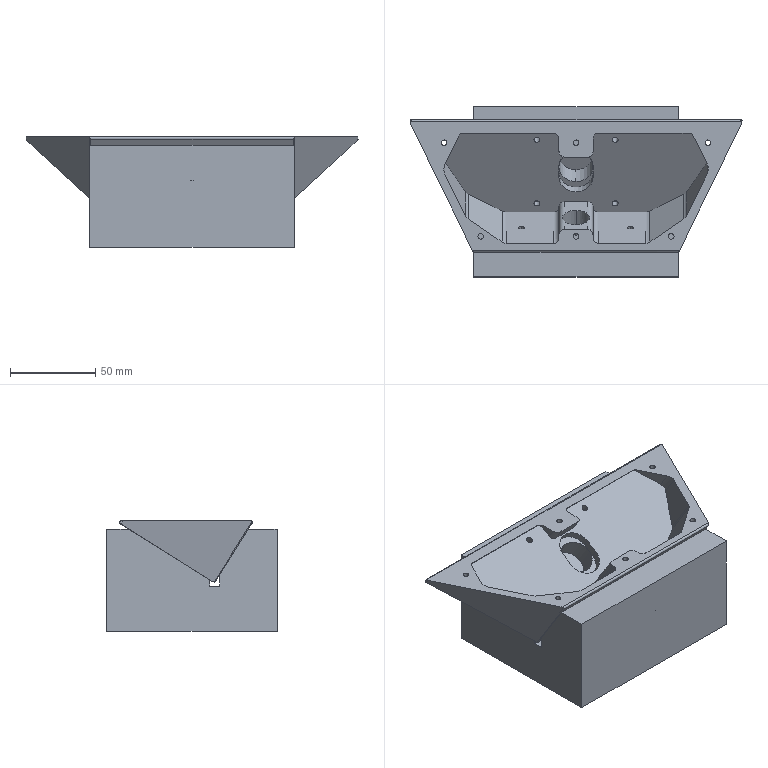NC program | Mastercam | posted with a generic post | part box 195.124 x 100 x 65 mm
Lines 1043 to 4164 of 16336, first 3080 of 3122 lines:
N440 T10 M6
N450 G0 G90 G17 G54 X-64. Y-36.8 A0. S5500 M3
N460 G43 H10 Z50.
N470 Z3.12
N480 G1 Z-1.88 F2000.
N490 X-60. F3500.
N500 X60.
N510 X64.
N520 Y-36.721
N530 Z-2.007
N540 X60.
N550 X-60.
N560 X-64.
N570 Y-36.642
N580 Z-2.134
N590 X-60.
N600 X60.
N610 X64.
N620 Y-36.562
N630 Z-2.261
N640 X60.
N650 X-60.
N660 X-64.
N670 Y-36.483
N680 Z-2.388
N690 X-60.
N700 X60.
N710 X64.
N720 Y-36.404
N730 Z-2.515
N740 X60.
N750 X-60.
N760 X-64.
N770 Y-36.325
N780 Z-2.642
N790 X-60.
N800 X60.
N810 X64.
N820 Y-36.245
N830 Z-2.768
N840 X60.
N850 X-60.
N860 X-64.
N870 Y-36.166
N880 Z-2.895
N890 X-60.
N900 X60.
N910 X64.
N920 Y-36.087
N930 Z-3.022
N940 X60.
N950 X-60.
N960 X-64.
N970 Y-36.007
N980 Z-3.149
N990 X-60.
N1000 X60.
N1010 X64.
N1020 Y-35.928
N1030 Z-3.276
N1040 X60.
N1050 X-60.
N1060 X-64.
N1070 Y-35.849
N1080 Z-3.403
N1090 X-60.
N1100 X60.
N1110 X64.
N1120 Y-35.77
N1130 Z-3.53
N1140 X60.
N1150 X-60.
N1160 X-64.
N1170 Y-35.69
N1180 Z-3.657
N1190 X-60.
N1200 X60.
N1210 X64.
N1220 Y-35.611
N1230 Z-3.784
N1240 X60.
N1250 X-60.
N1260 X-64.
N1270 Y-35.532
N1280 Z-3.91
N1290 X-60.
N1300 X60.
N1310 X64.
N1320 Y-35.453
N1330 Z-4.037
N1340 X60.
N1350 X-60.
N1360 X-64.
N1370 Y-35.373
N1380 Z-4.164
N1390 X-60.
N1400 X60.
N1410 X64.
N1420 Y-35.294
N1430 Z-4.291
N1440 X60.
N1450 X-60.
N1460 X-64.
N1470 Y-35.215
N1480 Z-4.418
N1490 X-60.
N1500 X60.
N1510 X64.
N1520 Y-35.135
N1530 Z-4.545
N1540 X60.
N1550 X-60.
N1560 X-64.
N1570 Y-35.056
N1580 Z-4.672
N1590 X-60.
N1600 X60.
N1610 X64.
N1620 Y-34.977
N1630 Z-4.799
N1640 X60.
N1650 X-60.
N1660 X-64.
N1670 Y-34.898
N1680 Z-4.925
N1690 X-60.
N1700 X60.
N1710 X64.
N1720 Y-34.818
N1730 Z-5.052
N1740 X60.
N1750 X-60.
N1760 X-64.
N1770 Y-34.739
N1780 Z-5.179
N1790 X-60.
N1800 X60.
N1810 X64.
N1820 Y-34.66
N1830 Z-5.306
N1840 X60.
N1850 X-60.
N1860 X-64.
N1870 Y-34.58
N1880 Z-5.433
N1890 X-60.
N1900 X60.
N1910 X64.
N1920 Y-34.501
N1930 Z-5.56
N1940 X60.
N1950 X-60.
N1960 X-64.
N1970 Y-34.422
N1980 Z-5.687
N1990 X-60.
N2000 X60.
N2010 X64.
N2020 Y-34.343
N2030 Z-5.814
N2040 X60.
N2050 X-60.
N2060 X-64.
N2070 Y-34.263
N2080 Z-5.94
N2090 X-60.
N2100 X60.
N2110 X64.
N2120 Y-34.184
N2130 Z-6.067
N2140 X60.
N2150 X-60.
N2160 X-64.
N2170 Y-34.105
N2180 Z-6.194
N2190 X-60.
N2200 X60.
N2210 X64.
N2220 Y-34.025
N2230 Z-6.321
N2240 X60.
N2250 X-60.
N2260 X-64.
N2270 Y-33.946
N2280 Z-6.448
N2290 X-60.
N2300 X60.
N2310 X64.
N2320 Y-33.867
N2330 Z-6.575
N2340 X60.
N2350 X-60.
N2360 X-64.
N2370 Y-33.788
N2380 Z-6.702
N2390 X-60.
N2400 X60.
N2410 X64.
N2420 Y-33.708
N2430 Z-6.829
N2440 X60.
N2450 X-60.
N2460 X-64.
N2470 Y-33.629
N2480 Z-6.955
N2490 X-60.
N2500 X60.
N2510 X64.
N2520 Y-33.55
N2530 Z-7.082
N2540 X60.
N2550 X-60.
N2560 X-64.
N2570 Y-33.47
N2580 Z-7.209
N2590 X-60.
N2600 X60.
N2610 X64.
N2620 Y-33.391
N2630 Z-7.336
N2640 X60.
N2650 X-60.
N2660 X-64.
N2670 Y-33.312
N2680 Z-7.463
N2690 X-60.
N2700 X60.
N2710 X64.
N2720 Y-33.233
N2730 Z-7.59
N2740 X60.
N2750 X-60.
N2760 X-64.
N2770 Y-33.153
N2780 Z-7.717
N2790 X-60.
N2800 X60.
N2810 X64.
N2820 Y-33.074
N2830 Z-7.844
N2840 X60.
N2850 X-60.
N2860 X-64.
N2870 Y-32.995
N2880 Z-7.971
N2890 X-60.
N2900 X60.
N2910 X64.
N2920 Y-32.915
N2930 Z-8.097
N2940 X60.
N2950 X-60.
N2960 X-64.
N2970 Y-32.836
N2980 Z-8.224
N2990 X-60.
N3000 X60.
N3010 X64.
N3020 Y-32.757
N3030 Z-8.351
N3040 X60.
N3050 X-60.
N3060 X-64.
N3070 Y-32.678
N3080 Z-8.478
N3090 X-60.
N3100 X60.
N3110 X64.
N3120 Y-32.598
N3130 Z-8.605
N3140 X60.
N3150 X-60.
N3160 X-64.
N3170 Y-32.519
N3180 Z-8.732
N3190 X-60.
N3200 X60.
N3210 X64.
N3220 Y-32.44
N3230 Z-8.859
N3240 X60.
N3250 X-60.
N3260 X-64.
N3270 Y-32.36
N3280 Z-8.986
N3290 X-60.
N3300 X60.
N3310 X64.
N3320 Y-32.281
N3330 Z-9.112
N3340 X60.
N3350 X-60.
N3360 X-64.
N3370 Y-32.202
N3380 Z-9.239
N3390 X-60.
N3400 X60.
N3410 X64.
N3420 Y-32.123
N3430 Z-9.366
N3440 X60.
N3450 X-60.
N3460 X-64.
N3470 Y-32.043
N3480 Z-9.493
N3490 X-60.
N3500 X60.
N3510 X64.
N3520 Y-31.964
N3530 Z-9.62
N3540 X60.
N3550 X-60.
N3560 X-64.
N3570 Y-31.885
N3580 Z-9.747
N3590 X-60.
N3600 X60.
N3610 X64.
N3620 Y-31.805
N3630 Z-9.874
N3640 X60.
N3650 X-60.
N3660 X-64.
N3670 Y-31.726
N3680 Z-10.001
N3690 X-60.
N3700 X60.
N3710 X64.
N3720 Y-31.647
N3730 Z-10.127
N3740 X60.
N3750 X-60.
N3760 X-64.
N3770 Y-31.568
N3780 Z-10.254
N3790 X-60.
N3800 X60.
N3810 X64.
N3820 Y-31.488
N3830 Z-10.381
N3840 X60.
N3850 X-60.
N3860 X-64.
N3870 Y-31.409
N3880 Z-10.508
N3890 X-60.
N3900 X60.
N3910 X64.
N3920 Y-31.33
N3930 Z-10.635
N3940 X60.
N3950 X-60.
N3960 X-64.
N3970 Y-31.251
N3980 Z-10.762
N3990 X-60.
N4000 X60.
N4010 X64.
N4020 Y-31.171
N4030 Z-10.889
N4040 X60.
N4050 X-60.
N4060 X-64.
N4070 Y-31.092
N4080 Z-11.016
N4090 X-60.
N4100 X60.
N4110 X64.
N4120 Y-31.013
N4130 Z-11.143
N4140 X60.
N4150 X-60.
N4160 X-64.
N4170 Y-30.933
N4180 Z-11.269
N4190 X-60.
N4200 X60.
N4210 X64.
N4220 Y-30.854
N4230 Z-11.396
N4240 X60.
N4250 X-60.
N4260 X-64.
N4270 Y-30.775
N4280 Z-11.523
N4290 X-60.
N4300 X60.
N4310 X64.
N4320 Y-30.696
N4330 Z-11.65
N4340 X60.
N4350 X-60.
N4360 X-64.
N4370 Y-30.616
N4380 Z-11.777
N4390 X-60.
N4400 X60.
N4410 X64.
N4420 Y-30.537
N4430 Z-11.904
N4440 X60.
N4450 X-60.
N4460 X-64.
N4470 Y-30.458
N4480 Z-12.031
N4490 X-60.
N4500 X60.
N4510 X64.
N4520 Y-30.378
N4530 Z-12.158
N4540 X60.
N4550 X-60.
N4560 X-64.
N4570 Y-30.299
N4580 Z-12.284
N4590 X-60.
N4600 X60.
N4610 X64.
N4620 Y-30.22
N4630 Z-12.411
N4640 X60.
N4650 X-60.
N4660 X-64.
N4670 Y-30.141
N4680 Z-12.538
N4690 X-60.
N4700 X60.
N4710 X64.
N4720 Y-30.061
N4730 Z-12.665
N4740 X60.
N4750 X-60.
N4760 X-64.
N4770 Y-29.982
N4780 Z-12.792
N4790 X-60.
N4800 X60.
N4810 X64.
N4820 Y-29.903
N4830 Z-12.919
N4840 X60.
N4850 X-60.
N4860 X-64.
N4870 Y-29.823
N4880 Z-13.046
N4890 X-60.
N4900 X60.
N4910 X64.
N4920 Y-29.744
N4930 Z-13.173
N4940 X60.
N4950 X-60.
N4960 X-64.
N4970 Y-29.665
N4980 Z-13.299
N4990 X-60.
N5000 X60.
N5010 X64.
N5020 Y-29.586
N5030 Z-13.426
N5040 X60.
N5050 X-60.
N5060 X-64.
N5070 Y-29.506
N5080 Z-13.553
N5090 X-60.
N5100 X60.
N5110 X64.
N5120 Y-29.427
N5130 Z-13.68
N5140 X60.
N5150 X-60.
N5160 X-64.
N5170 Y-29.348
N5180 Z-13.807
N5190 X-60.
N5200 X60.
N5210 X64.
N5220 Y-29.268
N5230 Z-13.934
N5240 X60.
N5250 X-60.
N5260 X-64.
N5270 Y-29.189
N5280 Z-14.061
N5290 X-60.
N5300 X60.
N5310 X64.
N5320 Y-29.11
N5330 Z-14.188
N5340 X60.
N5350 X-60.
N5360 X-64.
N5370 Y-29.031
N5380 Z-14.314
N5390 X-60.
N5400 X60.
N5410 X64.
N5420 Y-28.951
N5430 Z-14.441
N5440 X60.
N5450 X-60.
N5460 X-64.
N5470 Y-28.872
N5480 Z-14.568
N5490 X-60.
N5500 X60.
N5510 X64.
N5520 Y-28.793
N5530 Z-14.695
N5540 X60.
N5550 X-60.
N5560 X-64.
N5570 Y-28.713
N5580 Z-14.822
N5590 X-60.
N5600 X60.
N5610 X64.
N5620 Y-28.634
N5630 Z-14.949
N5640 X60.
N5650 X-60.
N5660 X-64.
N5670 Y-28.555
N5680 Z-15.076
N5690 X-60.
N5700 X60.
N5710 X64.
N5720 Y-28.476
N5730 Z-15.203
N5740 X60.
N5750 X-60.
N5760 X-64.
N5770 Y-28.396
N5780 Z-15.33
N5790 X-60.
N5800 X60.
N5810 X64.
N5820 Y-28.317
N5830 Z-15.456
N5840 X60.
N5850 X-60.
N5860 X-64.
N5870 Y-28.238
N5880 Z-15.583
N5890 X-60.
N5900 X60.
N5910 X64.
N5920 Y-28.158
N5930 Z-15.71
N5940 X60.
N5950 X-60.
N5960 X-64.
N5970 Y-28.079
N5980 Z-15.837
N5990 X-60.
N6000 X60.
N6010 X64.
N6020 Y-28.
N6030 Z-15.964
N6040 X60.
N6050 X-60.
N6060 X-64.
N6070 Y-27.921
N6080 Z-16.091
N6090 X-60.
N6100 X60.
N6110 X64.
N6120 Y-27.841
N6130 Z-16.218
N6140 X60.
N6150 X-60.
N6160 X-64.
N6170 Y-27.762
N6180 Z-16.345
N6190 X-60.
N6200 X60.
N6210 X64.
N6220 Y-27.683
N6230 Z-16.471
N6240 X60.
N6250 X-60.
N6260 X-64.
N6270 Y-27.603
N6280 Z-16.598
N6290 X-60.
N6300 X60.
N6310 X64.
N6320 Y-27.524
N6330 Z-16.725
N6340 X60.
N6350 X-60.
N6360 X-64.
N6370 Y-27.445
N6380 Z-16.852
N6390 X-60.
N6400 X60.
N6410 X64.
N6420 Y-27.366
N6430 Z-16.979
N6440 X60.
N6450 X-60.
N6460 X-64.
N6470 Y-27.286
N6480 Z-17.106
N6490 X-60.
N6500 X60.
N6510 X64.
N6520 Y-27.207
N6530 Z-17.233
N6540 X60.
N6550 X-60.
N6560 X-64.
N6570 Y-27.128
N6580 Z-17.36
N6590 X-60.
N6600 X60.
N6610 X64.
N6620 Y-27.049
N6630 Z-17.486
N6640 X60.
N6650 X-60.
N6660 X-64.
N6670 Y-26.969
N6680 Z-17.613
N6690 X-60.
N6700 X60.
N6710 X64.
N6720 Y-26.89
N6730 Z-17.74
N6740 X60.
N6750 X-60.
N6760 X-64.
N6770 Y-26.811
N6780 Z-17.867
N6790 X-60.
N6800 X60.
N6810 X64.
N6820 Y-26.731
N6830 Z-17.994
N6840 X60.
N6850 X-60.
N6860 X-64.
N6870 Y-26.652
N6880 Z-18.121
N6890 X-60.
N6900 X60.
N6910 X64.
N6920 Y-26.573
N6930 Z-18.248
N6940 X60.
N6950 X-60.
N6960 X-64.
N6970 Y-26.494
N6980 Z-18.375
N6990 X-60.
N7000 X60.
N7010 X64.
N7020 Y-26.414
N7030 Z-18.502
N7040 X60.
N7050 X-60.
N7060 X-64.
N7070 Y-26.335
N7080 Z-18.628
N7090 X-60.
N7100 X60.
N7110 X64.
N7120 Y-26.256
N7130 Z-18.755
N7140 X60.
N7150 X-60.
N7160 X-64.
N7170 Y-26.176
N7180 Z-18.882
N7190 X-60.
N7200 X60.
N7210 X64.
N7220 Y-26.097
N7230 Z-19.009
N7240 X60.
N7250 X-60.
N7260 X-64.
N7270 Y-26.018
N7280 Z-19.136
N7290 X-60.
N7300 X60.
N7310 X64.
N7320 Y-25.939
N7330 Z-19.263
N7340 X60.
N7350 X-60.
N7360 X-64.
N7370 Y-25.859
N7380 Z-19.39
N7390 X-60.
N7400 X60.
N7410 X64.
N7420 Y-25.78
N7430 Z-19.517
N7440 X60.
N7450 X-60.
N7460 X-64.
N7470 Y-25.701
N7480 Z-19.643
N7490 X-60.
N7500 X60.
N7510 X64.
N7520 Y-25.621
N7530 Z-19.77
N7540 X60.
N7550 X-60.
N7560 X-64.
N7570 Y-25.542
N7580 Z-19.897
N7590 X-60.
N7600 X60.
N7610 X64.
N7620 Y-25.463
N7630 Z-20.024
N7640 X60.
N7650 X-60.
N7660 X-64.
N7670 Y-25.384
N7680 Z-20.151
N7690 X-60.
N7700 X60.
N7710 X64.
N7720 Y-25.304
N7730 Z-20.278
N7740 X60.
N7750 X-60.
N7760 X-64.
N7770 Y-25.225
N7780 Z-20.405
N7790 X-60.
N7800 X60.
N7810 X64.
N7820 Y-25.146
N7830 Z-20.532
N7840 X60.
N7850 X-60.
N7860 X-64.
N7870 Y-25.066
N7880 Z-20.658
N7890 X-60.
N7900 X60.
N7910 X64.
N7920 Y-24.987
N7930 Z-20.785
N7940 X60.
N7950 X-60.
N7960 X-64.
N7970 Y-24.908
N7980 Z-20.912
N7990 X-60.
N8000 X60.
N8010 X64.
N8020 Y-24.829
N8030 Z-21.039
N8040 X60.
N8050 X-60.
N8060 X-64.
N8070 Y-24.749
N8080 Z-21.166
N8090 X-60.
N8100 X60.
N8110 X64.
N8120 Y-24.67
N8130 Z-21.293
N8140 X60.
N8150 X-60.
N8160 X-64.
N8170 Y-24.591
N8180 Z-21.42
N8190 X-60.
N8200 X60.
N8210 X64.
N8220 Y-24.511
N8230 Z-21.547
N8240 X60.
N8250 X-60.
N8260 X-64.
N8270 Y-24.432
N8280 Z-21.673
N8290 X-60.
N8300 X60.
N8310 X64.
N8320 Y-24.353
N8330 Z-21.8
N8340 X60.
N8350 X-60.
N8360 X-64.
N8370 Y-24.274
N8380 Z-21.927
N8390 X-60.
N8400 X60.
N8410 X64.
N8420 Y-24.194
N8430 Z-22.054
N8440 X60.
N8450 X-60.
N8460 X-64.
N8470 Y-24.115
N8480 Z-22.181
N8490 X-60.
N8500 X60.
N8510 X64.
N8520 Y-24.036
N8530 Z-22.308
N8540 X60.
N8550 X-60.
N8560 X-64.
N8570 Y-23.956
N8580 Z-22.435
N8590 X-60.
N8600 X60.
N8610 X64.
N8620 Y-23.877
N8630 Z-22.562
N8640 X60.
N8650 X-60.
N8660 X-64.
N8670 Y-23.798
N8680 Z-22.689
N8690 X-60.
N8700 X60.
N8710 X64.
N8720 Y-23.719
N8730 Z-22.815
N8740 X60.
N8750 X-60.
N8760 X-64.
N8770 Y-23.639
N8780 Z-22.942
N8790 X-60.
N8800 X60.
N8810 X64.
N8820 Y-23.56
N8830 Z-23.069
N8840 X60.
N8850 X-60.
N8860 X-64.
N8870 Y-23.481
N8880 Z-23.196
N8890 X-60.
N8900 X60.
N8910 X64.
N8920 Y-23.401
N8930 Z-23.323
N8940 X60.
N8950 X-60.
N8960 X-64.
N8970 Y-23.322
N8980 Z-23.45
N8990 X-60.
N9000 X60.
N9010 X64.
N9020 Y-23.243
N9030 Z-23.577
N9040 X60.
N9050 X-60.
N9060 X-64.
N9070 Y-23.164
N9080 Z-23.704
N9090 X-60.
N9100 X60.
N9110 X64.
N9120 Y-23.084
N9130 Z-23.83
N9140 X60.
N9150 X-60.
N9160 X-64.
N9170 Y-23.005
N9180 Z-23.957
N9190 X-60.
N9200 X60.
N9210 X64.
N9220 Y-22.926
N9230 Z-24.084
N9240 X60.
N9250 X-60.
N9260 X-64.
N9270 Y-22.847
N9280 Z-24.211
N9290 X-60.
N9300 X60.
N9310 X64.
N9320 Y-22.767
N9330 Z-24.338
N9340 X60.
N9350 X-60.
N9360 X-64.
N9370 Y-22.688
N9380 Z-24.465
N9390 X-60.
N9400 X60.
N9410 X64.
N9420 Y-22.609
N9430 Z-24.592
N9440 X60.
N9450 X-60.
N9460 X-64.
N9470 Y-22.529
N9480 Z-24.719
N9490 X-60.
N9500 X60.
N9510 X64.
N9520 Y-22.45
N9530 Z-24.845
N9540 X60.
N9550 X-60.
N9560 X-64.
N9570 Y-22.371
N9580 Z-24.972
N9590 X-60.
N9600 X60.
N9610 X64.
N9620 Y-22.292
N9630 Z-25.099
N9640 X60.
N9650 X-60.
N9660 X-64.
N9670 Y-22.212
N9680 Z-25.226
N9690 X-60.
N9700 X60.
N9710 X64.
N9720 Y-22.133
N9730 Z-25.353
N9740 X60.
N9750 X-60.
N9760 X-64.
N9770 Y-22.054
N9780 Z-25.48
N9790 X-60.
N9800 X60.
N9810 X64.
N9820 Y-21.974
N9830 Z-25.607
N9840 X60.
N9850 X-60.
N9860 X-64.
N9870 Y-21.895
N9880 Z-25.734
N9890 X-60.
N9900 X60.
N9910 X64.
N9920 Y-21.816
N9930 Z-25.861
N9940 X60.
N9950 X-60.
N9960 X-64.
N9970 Y-21.737
N9980 Z-25.987
N9990 X-60.
N100 X60.
N110 X64.
N120 Y-21.657
N130 Z-26.114
N140 X60.
N150 X-60.
N160 X-64.
N170 Y-21.578
N180 Z-26.241
N190 X-60.
N200 X60.
N210 X64.
N220 Y-21.499
N230 Z-26.368
N240 X60.
N250 X-60.
N260 X-64.
N270 Y-21.419
N280 Z-26.495
N290 X-60.
N300 X60.
N310 X64.
N320 Y-21.34
N330 Z-26.622
N340 X60.
N350 X-60.
N360 X-64.
N370 Y-21.261
N380 Z-26.749
N390 X-60.
N400 X60.
N410 X64.
N420 Y-21.182
N430 Z-26.876
N440 X60.
N450 X-60.
N460 X-64.
N470 Y-21.102
N480 Z-27.002
N490 X-60.
N500 X60.
N510 X64.
N520 Y-21.023
N530 Z-27.129
N540 X60.
N550 X-60.
N560 X-64.
N570 Y-20.944
N580 Z-27.256
N590 X-60.
N600 X60.
N610 X64.
N620 Y-20.864
N630 Z-27.383
N640 X60.
N650 X-60.
N660 X-64.
N670 Y-20.785
N680 Z-27.51
N690 X-60.
N700 X60.
N710 X64.
N720 Y-20.706
N730 Z-27.637
N740 X60.
N750 X-60.
N760 X-64.
N770 Y-20.627
N780 Z-27.764
N790 X-60.
N800 X60.
N810 X64.
N820 Y-20.547
N830 Z-27.891
N840 X60.
N850 X-60.
N860 X-64.
N870 Y-20.468
N880 Z-28.017
N890 X-60.
N900 X60.
N910 X64.
N920 Y-20.389
N930 Z-28.144
N940 X60.
N950 X-60.
N960 X-64.
N970 Y-20.309
N980 Z-28.271
N990 X-60.
N1000 X60.
N1010 X64.
N1020 Y-20.23
N1030 Z-28.398
N1040 X60.
N1050 X-60.
N1060 X-64.
N1070 Y-20.151
N1080 Z-28.525
N1090 X-60.
N1100 X60.
N1110 X64.
N1120 Y-20.072
N1130 Z-28.652
N1140 X60.
N1150 X-60.
N1160 X-64.
N1170 Y-19.992
N1180 Z-28.779
N1190 X-60.
N1200 X60.
N1210 X64.
N1220 Y-19.913
N1230 Z-28.906
N1240 X60.
N1250 X-60.
N1260 X-64.
N1270 Y-19.834
N1280 Z-29.032
N1290 X-60.
N1300 X60.
N1310 X64.
N1320 Y-19.754
N1330 Z-29.159
N1340 X60.
N1350 X-60.
N1360 X-64.
N1370 Y-19.675
N1380 Z-29.286
N1390 X-60.
N1400 X60.
N1410 X64.
N1420 Y-19.596
N1430 Z-29.413
N1440 X60.
N1450 X-60.
N1460 X-64.
N1470 Y-19.517
N1480 Z-29.54
N1490 X-60.
N1500 X60.
N1510 X64.
N1520 Y-19.437
N1530 Z-29.667
N1540 X60.
N1550 X-60.
N1560 X-64.
N1570 Y-19.358
N1580 Z-29.794
N1590 X-60.
N1600 X60.
N1610 X64.
N1620 Y-19.279
N1630 Z-29.921
N1640 X60.
N1650 X-60.
N1660 X-64.
N1670 Y-19.217
N1680 Z-29.928
N1690 X-60.
N1700 X60.
N1710 X64.
N1720 Z-29.849
N1730 Y-19.089
N1740 X60.
N1750 X-60.
N1760 X-64.
N1770 Z-29.77
N1780 Y-18.962
N1790 X-60.
N1800 X60.
N1810 X64.
N1820 Z-29.69
N1830 Y-18.835
N1840 X60.
N1850 X-60.
N1860 X-64.
N1870 Z-29.611
N1880 Y-18.708
N1890 X-60.
N1900 X60.
N1910 X64.
N1920 Z-29.531
N1930 Y-18.581
N1940 X60.
N1950 X-60.
N1960 X-64.
N1970 Z-29.452
N1980 Y-18.454
N1990 X-60.
N2000 X60.
N2010 X64.
N2020 Z-29.372
N2030 Y-18.326
N2040 X60.
N2050 X-60.
N2060 X-64.
N2070 Z-29.293
N2080 Y-18.199
N2090 X-60.
N2100 X60.
N2110 X64.
N2120 Z-29.213
N2130 Y-18.072
N2140 X60.
N2150 X-60.
N2160 X-64.
N2170 Z-29.134
N2180 Y-17.945
N2190 X-60.
N2200 X60.
N2210 X64.
N2220 Z-29.054
N2230 Y-17.818
N2240 X60.
N2250 X-60.
N2260 X-64.
N2270 Z-28.975
N2280 Y-17.691
N2290 X-60.
N2300 X60.
N2310 X64.
N2320 Z-28.895
N2330 Y-17.564
N2340 X60.
N2350 X-60.
N2360 X-64.
N2370 Z-28.816
N2380 Y-17.436
N2390 X-60.
N2400 X60.
N2410 X64.
N2420 Z-28.737
N2430 Y-17.309
N2440 X60.
N2450 X-60.
N2460 X-64.
N2470 Z-28.657
N2480 Y-17.182
N2490 X-60.
N2500 X60.
N2510 X64.
N2520 Z-28.578
N2530 Y-17.055
N2540 X60.
N2550 X-60.
N2560 X-64.
N2570 Z-28.498
N2580 Y-16.928
N2590 X-60.
N2600 X60.
N2610 X64.
N2620 Z-28.419
N2630 Y-16.801
N2640 X60.
N2650 X-60.
N2660 X-64.
N2670 Z-28.339
N2680 Y-16.673
N2690 X-60.
N2700 X60.
N2710 X64.
N2720 Z-28.26
N2730 Y-16.546
N2740 X60.
N2750 X-60.
N2760 X-64.
N2770 Z-28.18
N2780 Y-16.419
N2790 X-60.
N2800 X60.
N2810 X64.
N2820 Z-28.101
N2830 Y-16.292
N2840 X60.
N2850 X-60.
N2860 X-64.
N2870 Z-28.021
N2880 Y-16.165
N2890 X-60.
N2900 X60.
N2910 X64.
N2920 Z-27.942
N2930 Y-16.038
N2940 X60.
N2950 X-60.
N2960 X-64.
N2970 Z-27.863
N2980 Y-15.91
N2990 X-60.
N3000 X60.
N3010 X64.
N3020 Z-27.783
N3030 Y-15.783
N3040 X60.
N3050 X-60.
N3060 X-64.
N3070 Z-27.704
N3080 Y-15.656
N3090 X-60.
N3100 X60.
N3110 X64.
N3120 Z-27.624
N3130 Y-15.529
N3140 X60.
N3150 X-60.
N3160 X-64.
N3170 Z-27.545
N3180 Y-15.402
N3190 X-60.
N3200 X60.
N3210 X64.
N3220 Z-27.465
N3230 Y-15.275
N3240 X60.
N3250 X-60.
N3260 X-64.
N3270 Z-27.386
N3280 Y-15.147
N3290 X-60.
N3300 X60.
N3310 X64.
N3320 Z-27.306
N3330 Y-15.02
N3340 X60.
N3350 X-60.
N3360 X-64.
N3370 Z-27.227
N3380 Y-14.893
N3390 X-60.
N3400 X60.
N3410 X64.
N3420 Z-27.147
N3430 Y-14.766
N3440 X60.
N3450 X-60.
N3460 X-64.
N3470 Z-27.068
N3480 Y-14.639
N3490 X-60.
N3500 X60.
N3510 X64.
N3520 Z-26.988
N3530 Y-14.512
N3540 X60.
N3550 X-60.
N3560 X-64.
N3570 Z-26.909
N3580 Y-14.384
N3590 X-60.
N3600 X60.
N3610 X64.
N3620 Z-26.83
N3630 Y-14.257
N3640 X60.
N3650 X-60.
N3660 X-64.
N3670 Z-26.75
N3680 Y-14.13
N3690 X-60.
N3700 X60.
N3710 X64.
N3720 Z-26.671
N3730 Y-14.003
N3740 X60.
N3750 X-60.
N3760 X-64.
N3770 Z-26.591
N3780 Y-13.876
N3790 X-60.
N3800 X60.
N3810 X64.
N3820 Z-26.512
N3830 Y-13.749
N3840 X60.
N3850 X-60.
N3860 X-64.
N3870 Z-26.432
N3880 Y-13.621
N3890 X-60.
N3900 X60.
N3910 X64.
N3920 Z-26.353
N3930 Y-13.494
N3940 X60.
N3950 X-60.
N3960 X-64.
N3970 Z-26.273
N3980 Y-13.367
N3990 X-60.
N4000 X60.
N4010 X64.
N4020 Z-26.194
N4030 Y-13.24
N4040 X60.
N4050 X-60.
N4060 X-64.
N4070 Z-26.114
N4080 Y-13.113
N4090 X-60.
N4100 X60.
N4110 X64.
N4120 Z-26.035
N4130 Y-12.986
N4140 X60.
N4150 X-60.
N4160 X-64.
N4170 Z-25.955
N4180 Y-12.859
N4190 X-60.
N4200 X60.
N4210 X64.
N4220 Z-25.876
N4230 Y-12.731
N4240 X60.
N4250 X-60.
N4260 X-64.
N4270 Z-25.797
N4280 Y-12.604
N4290 X-60.
N4300 X60.
N4310 X64.
N4320 Z-25.717
N4330 Y-12.477
N4340 X60.
N4350 X-60.
N4360 X-64.
N4370 Z-25.638
N4380 Y-12.35
N4390 X-60.
N4400 X60.
N4410 X64.
N4420 Z-25.558
N4430 Y-12.223
N4440 X60.
N4450 X-60.
N4460 X-64.
N4470 Z-25.479
N4480 Y-12.096
N4490 X-60.
N4500 X60.
N4510 X64.
N4520 Z-25.399
N4530 Y-11.968
N4540 X60.
N4550 X-60.
N4560 X-64.
N4570 Z-25.32
N4580 Y-11.841
N4590 X-60.
N4600 X60.
N4610 X64.
N4620 Z-25.24
N4630 Y-11.714
N4640 X60.
N4650 X-60.
N4660 X-64.
N4670 Z-25.161
N4680 Y-11.587
N4690 X-60.
N4700 X60.
N4710 X64.
N4720 Z-25.081
N4730 Y-11.46
N4740 X60.
N4750 X-60.
N4760 X-64.
N4770 Z-25.002
N4780 Y-11.333
N4790 X-60.
N4800 X60.
N4810 X64.
N4820 Z-24.922
N4830 Y-11.205
N4840 X60.
N4850 X-60.
N4860 X-64.
N4870 Z-24.843
N4880 Y-11.078
N4890 X-60.
N4900 X60.
N4910 X64.
N4920 Z-24.764
N4930 Y-10.951
N4940 X60.
N4950 X-60.
N4960 X-64.
N4970 Z-24.684
N4980 Y-10.824
N4990 X-60.
N5000 X60.
N5010 X64.
N5020 Z-24.605
N5030 Y-10.697
N5040 X60.
N5050 X-60.
N5060 X-64.
N5070 Z-24.525
N5080 Y-10.57
N5090 X-60.
N5100 X60.
N5110 X64.
N5120 Z-24.446
N5130 Y-10.442
N5140 X60.
N5150 X-60.
N5160 X-64.
N5170 Z-24.366
N5180 Y-10.315
N5190 X-60.
N5200 X60.
N5210 X64.
N5220 Z-24.287
N5230 Y-10.188
N5240 X60.
N5250 X-60.
N5260 X-64.
N5270 Z-24.207
N5280 Y-10.061
N5290 X-60.
N5300 X60.
N5310 X64.
N5320 Z-24.128
N5330 Y-9.934
N5340 X60.
N5350 X-60.
N5360 X-64.
N5370 Z-24.048
N5380 Y-9.807
N5390 X-60.
N5400 X60.
N5410 X64.
N5420 Z-23.969
N5430 Y-9.679
N5440 X60.
N5450 X-60.
N5460 X-64.
N5470 Z-23.89
N5480 Y-9.552
N5490 X-60.
N5500 X60.
N5510 X64.
N5520 Z-23.81
N5530 Y-9.425
N5540 X60.
N5550 X-60.
N5560 X-64.
N5570 Z-23.731
N5580 Y-9.298
N5590 X-60.
N5600 X60.
N5610 X64.
N5620 Z-23.651
N5630 Y-9.171
N5640 X60.
N5650 X-60.
N5660 X-64.
N5670 Z-23.572
N5680 Y-9.044
N5690 X-60.
N5700 X60.
N5710 X64.
N5720 Z-23.492
N5730 Y-8.916
N5740 X60.
N5750 X-60.
N5760 X-64.
N5770 Z-23.413
N5780 Y-8.789
N5790 X-60.
N5800 X60.
N5810 X64.
N5820 Z-23.333
N5830 Y-8.662
N5840 X60.
N5850 X-60.
N5860 X-64.
N5870 Z-23.254
N5880 Y-8.535
N5890 X-60.
N5900 X60.
N5910 X64.
N5920 Z-23.174
N5930 Y-8.408
N5940 X60.
N5950 X-60.
N5960 X-64.
N5970 Z-23.095
N5980 Y-8.281
N5990 X-60.
N6000 X60.
N6010 X64.
N6020 Z-23.015
N6030 Y-8.154
N6040 X60.
N6050 X-60.
N6060 X-64.
N6070 Z-22.936
N6080 Y-8.026
N6090 X-60.
N6100 X60.
N6110 X64.
N6120 Z-22.857
N6130 Y-7.899
N6140 X60.
N6150 X-60.
N6160 X-64.
N6170 Z-22.777
N6180 Y-7.772
N6190 X-60.
N6200 X60.
N6210 X64.
N6220 Z-22.698
N6230 Y-7.645
N6240 X60.
N6250 X-60.
N6260 X-64.
N6270 Z-22.618
N6280 Y-7.518
N6290 X-60.
N6300 X60.
N6310 X64.
N6320 Z-22.539
N6330 Y-7.391
N6340 X60.
N6350 X-60.
N6360 X-64.
N6370 Z-22.459
N6380 Y-7.263
N6390 X-60.
N6400 X60.
N6410 X64.
N6420 Z-22.38
N6430 Y-7.136
N6440 X60.
N6450 X-60.
N6460 X-64.
N6470 Z-22.3
N6480 Y-7.009
N6490 X-60.
N6500 X60.
N6510 X64.
N6520 Z-22.221
N6530 Y-6.882
N6540 X60.
N6550 X-60.
N6560 X-64.
N6570 Z-22.141
N6580 Y-6.755
N6590 X-60.
N6600 X60.
N6610 X64.
N6620 Z-22.062
N6630 Y-6.628
N6640 X60.
N6650 X-60.
N6660 X-64.
N6670 Z-21.982
N6680 Y-6.5
N6690 X-60.
N6700 X60.
N6710 X64.
N6720 Z-21.903
N6730 Y-6.373
N6740 X60.
N6750 X-60.
N6760 X-64.
N6770 Z-21.824
N6780 Y-6.246
N6790 X-60.
N6800 X60.
N6810 X64.
N6820 Z-21.744
N6830 Y-6.119
N6840 X60.
N6850 X-60.
N6860 X-64.
N6870 Z-21.665
N6880 Y-5.992
N6890 X-60.
N6900 X60.
N6910 X64.
N6920 Z-21.585
N6930 Y-5.865
N6940 X60.
N6950 X-60.
N6960 X-64.
N6970 Z-21.506
N6980 Y-5.737
N6990 X-60.
N7000 X60.
N7010 X64.
N7020 Z-21.426
N7030 Y-5.61
N7040 X60.
N7050 X-60.
N7060 X-64.
N7070 Z-21.347
N7080 Y-5.483
N7090 X-60.
N7100 X60.
N7110 X64.
N7120 Z-21.267
N7130 Y-5.356
N7140 X60.
N7150 X-60.
N7160 X-64.
N7170 Z-21.188
N7180 Y-5.229
N7190 X-60.
N7200 X60.
N7210 X64.
N7220 Z-21.108
N7230 Y-5.102
N7240 X60.
N7250 X-60.
N7260 X-64.
N7270 Z-21.029
N7280 Y-4.974
N7290 X-60.
N7300 X60.
N7310 X64.
N7320 Z-20.95
N7330 Y-4.847
N7340 X60.
N7350 X-60.
N7360 X-64.
N7370 Z-20.87
N7380 Y-4.72
N7390 X-60.
N7400 X60.
N7410 X64.
N7420 Z-20.791
N7430 Y-4.593
N7440 X60.
N7450 X-60.
N7460 X-64.
N7470 Z-20.711
N7480 Y-4.466
N7490 X-60.
N7500 X60.
N7510 X64.
N7520 Z-20.632
N7530 Y-4.339
N7540 X60.
N7550 X-60.
N7560 X-64.
N7570 Z-20.552
N7580 Y-4.211
N7590 X-60.
N7600 X60.
N7610 X64.
N7620 Z-20.473
N7630 Y-4.084
N7640 X60.
N7650 X-60.
N7660 X-64.
N7670 Z-20.393
N7680 Y-3.957
N7690 X-60.
N7700 X60.
N7710 X64.
N7720 Z-20.314
N7730 Y-3.83
N7740 X60.
N7750 X-60.
N7760 X-64.
N7770 Z-20.234
N7780 Y-3.703
N7790 X-60.
N7800 X60.
N7810 X64.
N7820 Z-20.155
N7830 Y-3.576
N7840 X60.
N7850 X-60.
N7860 X-64.
N7870 Z-20.075
N7880 Y-3.449
N7890 X-60.
N7900 X60.
N7910 X64.
N7920 Z-19.996
N7930 Y-3.321
N7940 X60.
N7950 X-60.
N7960 X-64.
N7970 Z-19.917
N7980 Y-3.194
N7990 X-60.
N8000 X60.
N8010 X64.
N8020 Z-19.837
N8030 Y-3.067
N8040 X60.
N8050 X-60.
N8060 X-64.
N8070 Z-19.758
N8080 Y-2.94
N8090 X-60.
N8100 X60.
N8110 X64.
N8120 Z-19.678
N8130 Y-2.813
N8140 X60.
N8150 X-60.
N8160 X-64.
N8170 Z-19.599
N8180 Y-2.686
N8190 X-60.
N8200 X60.
N8210 X64.
N8220 Z-19.519
N8230 Y-2.558
N8240 X60.
N8250 X-60.
N8260 X-64.
N8270 Z-19.44
N8280 Y-2.431
N8290 X-60.
N8300 X60.
N8310 X64.
N8320 Z-19.36
N8330 Y-2.304
N8340 X60.
N8350 X-60.
N8360 X-64.
N8370 Z-19.281
N8380 Y-2.177
N8390 X-60.
N8400 X60.
N8410 X64.
N8420 Z-19.201
N8430 Y-2.05
N8440 X60.
N8450 X-60.
N8460 X-64.
N8470 Z-19.122
N8480 Y-1.923
N8490 X-60.
N8500 X60.
N8510 X64.
N8520 Z-19.042
N8530 Y-1.795
N8540 X60.
N8550 X-60.
N8560 X-64.
N8570 Z-18.963
N8580 Y-1.668
N8590 X-60.
N8600 X60.
N8610 X64.
N8620 Z-18.884
N8630 Y-1.541
N8640 X60.
N8650 X-60.
N8660 X-64.
N8670 Z-18.804
N8680 Y-1.414
N8690 X-60.
N8700 X60.
N8710 X64.
N8720 Z-18.725
N8730 Y-1.287
N8740 X60.
N8750 X-60.
N8760 X-64.
N8770 Z-18.645
N8780 Y-1.16
N8790 X-60.
N8800 X60.
N8810 X64.
N8820 Z-18.566
N8830 Y-1.032
N8840 X60.
N8850 X-60.
N8860 X-64.
N8870 Z-18.486
N8880 Y-.905
N8890 X-60.
N8900 X60.
N8910 X64.
N8920 Z-18.407
N8930 Y-.778
N8940 X60.
N8950 X-60.
N8960 X-64.
N8970 Z-18.327
N8980 Y-.651
N8990 X-60.
N9000 X60.
N9010 X64.
N9020 Z-18.248
N9030 Y-.524
N9040 X60.
N9050 X-60.
N9060 X-64.
N9070 Z-18.168
N9080 Y-.397
N9090 X-60.
N9100 X60.
N9110 X64.
N9120 Z-18.089
N9130 Y-.269
N9140 X60.
N9150 X-60.
N9160 X-64.
N9170 Z-18.009
N9180 Y-.142
N9190 X-60.
N9200 X60.
N9210 X64.
N9220 Z-17.93
N9230 Y-.015
N9240 X60.
N9250 X-60.
N9260 X-64.
N9270 Z-17.851
N9280 Y.112
N9290 X-60.
N9300 X60.
N9310 X64.
N9320 Z-17.771
N9330 Y.239
N9340 X60.
N9350 X-60.
N9360 X-64.
N9370 Z-17.692
N9380 Y.366
N9390 X-60.
N9400 X60.
N9410 X64.
N9420 Z-17.612
N9430 Y.494
N9440 X60.
N9450 X-60.
N9460 X-64.
N9470 Z-17.533
N9480 Y.621
N9490 X-60.
N9500 X60.
N9510 X64.
N9520 Z-17.453
N9530 Y.748
N9540 X60.
N9550 X-60.
N9560 X-64.
N9570 Z-17.374
N9580 Y.875
N9590 X-60.
N9600 X60.
N9610 X64.
N9620 Z-17.294
N9630 Y1.002
N9640 X60.
N9650 X-60.
N9660 X-64.
N9670 Z-17.215
N9680 Y1.129
N9690 X-60.
N9700 X60.
N9710 X64.
N9720 Z-17.135
N9730 Y1.256
N9740 X60.
N9750 X-60.
N9760 X-64.
N9770 Z-17.056
N9780 Y1.384
N9790 X-60.
N9800 X60.
N9810 X64.
N9820 Z-16.977
N9830 Y1.511
N9840 X60.
N9850 X-60.
N9860 X-64.
N9870 Z-16.897
N9880 Y1.638
N9890 X-60.
N9900 X60.
N9910 X64.
N9920 Z-16.818
N9930 Y1.765
N9940 X60.
N9950 X-60.
N9960 X-64.
N9970 Z-16.738
N9980 Y1.892
N9990 X-60.
N100 X60.
N110 X64.
N120 Z-16.659
N130 Y2.019
N140 X60.
N150 X-60.
N160 X-64.
N170 Z-16.579
N180 Y2.147
N190 X-60.
N200 X60.
N210 X64.
N220 Z-16.5
N230 Y2.274
N240 X60.
N250 X-60.
N260 X-64.
N270 Z-16.42
N280 Y2.401
N290 X-60.
N300 X60.
N310 X64.
N320 Z-16.341
N330 Y2.528
N340 X60.
N350 X-60.
N360 X-64.
N370 Z-16.261
N380 Y2.655
N390 X-60.
N400 X60.
N410 X64.
N420 Z-16.182
N430 Y2.782
N440 X60.
N450 X-60.
N460 X-64.
N470 Z-16.102
N480 Y2.91
N490 X-60.
N500 X60.
N510 X64.
N520 Z-16.023
N530 Y3.037
N540 X60.
N550 X-60.
N560 X-64.
N570 Z-15.944
N580 Y3.164
N590 X-60.
N600 X60.
N610 X64.
N620 Z-15.864
N630 Y3.291
N640 X60.
N650 X-60.
N660 X-64.
N670 Z-15.785
N680 Y3.418
N690 X-60.
N700 X60.
N710 X64.
N720 Z-15.705
N730 Y3.545
N740 X60.
N750 X-60.
N760 X-64.
N770 Z-15.626
N780 Y3.673
N790 X-60.
N800 X60.
N810 X64.
N820 Z-15.546
N830 Y3.8
N840 X60.
N850 X-60.
N860 X-64.
N870 Z-15.467
N880 Y3.927
N890 X-60.
N900 X60.
N910 X64.
N920 Z-15.387
N930 Y4.054
N940 X60.
N950 X-60.
N960 X-64.
N970 Z-15.308
N980 Y4.181
N990 X-60.
N1000 X60.
N1010 X64.
N1020 Z-15.228
N1030 Y4.308
N1040 X60.
N1050 X-60.
N1060 X-64.
N1070 Z-15.149
N1080 Y4.436
N1090 X-60.
N1100 X60.
N1110 X64.
N1120 Z-15.069
N1130 Y4.563
N1140 X60.
N1150 X-60.
N1160 X-64.
N1170 Z-14.99
N1180 Y4.69
N1190 X-60.
N1200 X60.
N1210 X64.
N1220 Z-14.911
N1230 Y4.817
N1240 X60.
N1250 X-60.
N1260 X-64.
N1270 Z-14.831
N1280 Y4.944
N1290 X-60.
N1300 X60.
N1310 X64.
N1320 Z-14.752
N1330 Y5.071
N1340 X60.
N1350 X-60.
N1360 X-64.
N1370 Z-14.672
N1380 Y5.199
N1390 X-60.
N1400 X60.
N1410 X64.
N1420 Z-14.593
N1430 Y5.326
N1440 X60.
N1450 X-60.
N1460 X-64.
N1470 Z-14.513
N1480 Y5.453
N1490 X-60.
N1500 X60.
N1510 X64.
N1520 Z-14.434
N1530 Y5.58
N1540 X60.
N1550 X-60.
N1560 X-64.
N1570 Z-14.354
N1580 Y5.707
N1590 X-60.
N1600 X60.
N1610 X64.
N1620 Z-14.275
N1630 Y5.834
N1640 X60.
N1650 X-60.
N1660 X-64.
N1670 Z-14.195
N1680 Y5.961
N1690 X-60.
N1700 X60.
N1710 X64.
N1720 Z-14.116
N1730 Y6.089
N1740 X60.
N1750 X-60.
N1760 X-64.
N1770 Z-14.037
N1780 Y6.216
N1790 X-60.
N1800 X60.
N1810 X64.
N1820 Z-13.957
N1830 Y6.343
N1840 X60.
N1850 X-60.
N1860 X-64.
N1870 Z-13.878
N1880 Y6.47
N1890 X-60.
N1900 X60.
N1910 X64.
N1920 Z-13.798
N1930 Y6.597
N1940 X60.
N1950 X-60.
N1960 X-64.
N1970 Z-13.719
N1980 Y6.724
N1990 X-60.
N2000 X60.
N2010 X64.
N2020 Z-13.639
N2030 Y6.852
N2040 X60.
N2050 X-60.
N2060 X-64.
N2070 Z-13.56
N2080 Y6.979
N2090 X-60.
N2100 X60.
N2110 X64.
N2120 Z-13.48
N2130 Y7.106
N2140 X60.
N2150 X-60.
N2160 X-64.
N2170 Z-13.401
N2180 Y7.233
N2190 X-60.
N2200 X60.
N2210 X64.
N2220 Z-13.321
N2230 Y7.36
N2240 X60.
N2250 X-60.
N2260 X-64.
N2270 Z-13.242
N2280 Y7.487
N2290 X-60.
N2300 X60.
N2310 X64.
N2320 Z-13.162
N2330 Y7.615
N2340 X60.
N2350 X-60.
N2360 X-64.
N2370 Z-13.083
N2380 Y7.742
N2390 X-60.
N2400 X60.
N2410 X64.
N2420 Z-13.004
N2430 Y7.869
N2440 X60.
N2450 X-60.
N2460 X-64.
N2470 Z-12.924
N2480 Y7.996
N2490 X-60.
N2500 X60.
N2510 X64.
N2520 Z-12.845
N2530 Y8.123
N2540 X60.
N2550 X-60.
N2560 X-64.
N2570 Z-12.765
N2580 Y8.25
N2590 X-60.
N2600 X60.
N2610 X64.
N2620 Z-12.686
N2630 Y8.378
N2640 X60.
N2650 X-60.
N2660 X-64.
N2670 Z-12.606
N2680 Y8.505
N2690 X-60.
N2700 X60.
N2710 X64.
N2720 Z-12.527
N2730 Y8.632
N2740 X60.
N2750 X-60.
N2760 X-64.
N2770 Z-12.447
N2780 Y8.759
N2790 X-60.
N2800 X60.
N2810 X64.
N2820 Z-12.368
N2830 Y8.886
N2840 X60.
N2850 X-60.
N2860 X-64.
N2870 Z-12.288
N2880 Y9.013
N2890 X-60.
N2900 X60.
N2910 X64.
N2920 Z-12.209
N2930 Y9.141
N2940 X60.
N2950 X-60.
N2960 X-64.
N2970 Z-12.129
N2980 Y9.268
N2990 X-60.
N3000 X60.
N3010 X64.
N3020 Z-12.05
N3030 Y9.395
N3040 X60.
N3050 X-60.
N3060 X-64.
N3070 Z-11.971
N3080 Y9.522
N3090 X-60.
N3100 X60.
N3110 X64.
N3120 Z-11.891
N3130 Y9.649
N3140 X60.
N3150 X-60.
N3160 X-64.
N3170 Z-11.812
N3180 Y9.776
N3190 X-60.
N3200 X60.
N3210 X64.
N3220 Z-11.732
N3230 Y9.904
N3240 X60.
N3250 X-60.
N3260 X-64.
N3270 Z-11.653
N3280 Y10.031
N3290 X-60.
N3300 X60.
N3310 X64.
N3320 Z-11.573
N3330 Y10.158
N3340 X60.
N3350 X-60.
N3360 X-64.
N3370 Z-11.494
N3380 Y10.285
N3390 X-60.
N3400 X60.
N3410 X64.
N3420 Z-11.414
N3430 Y10.412
N3440 X60.
N3450 X-60.
N3460 X-64.
N3470 Z-11.335
N3480 Y10.539
N3490 X-60.
N3500 X60.
N3510 X64.
N3520 Z-11.255
N3530 Y10.666
N3540 X60.
N3550 X-60.
N3560 X-64.
N3570 Z-11.176
N3580 Y10.794
N3590 X-60.
N3600 X60.
N3610 X64.
N3620 Z-11.096
N3630 Y10.921
N3640 X60.
N3650 X-60.
N3660 X-64.
N3670 Z-11.017
N3680 Y11.048
N3690 X-60.
N3700 X60.
N3710 X64.
N3720 Z-10.938
N3730 Y11.175
N3740 X60.
N3750 X-60.
N3760 X-64.
N3770 Z-10.858
N3780 Y11.302
N3790 X-60.
N3800 X60.
N3810 X64.
N3820 Z-10.779
N3830 Y11.429
N3840 X60.
N3850 X-60.
N3860 X-64.
N3870 Z-10.699
N3880 Y11.557
N3890 X-60.
N3900 X60.
N3910 X64.
N3920 Z-10.62
N3930 Y11.684
N3940 X60.
N3950 X-60.
N3960 X-64.
N3970 Z-10.54
N3980 Y11.811
N3990 X-60.
N4000 X60.
N4010 X64.
N4020 Z-10.461
N4030 Y11.938
N4040 X60.
N4050 X-60.
N4060 X-64.
N4070 Z-10.381
N4080 Y12.065
N4090 X-60.
N4100 X60.
N4110 X64.
N4120 Z-10.302
N4130 Y12.192
N4140 X60.
N4150 X-60.
N4160 X-64.
N4170 Z-10.222
N4180 Y12.32
N4190 X-60.
N4200 X60.
N4210 X64.
N4220 Z-10.143
N4230 Y12.447
N4240 X60.
N4250 X-60.
N4260 X-64.
N4270 Z-10.064
N4280 Y12.574
N4290 X-60.
N4300 X60.
N4310 X64.
N4320 Z-9.984
N4330 Y12.701
N4340 X60.
N4350 X-60.
N4360 X-64.
N4370 Z-9.905
N4380 Y12.828
N4390 X-60.
N4400 X60.
N4410 X64.
N4420 Z-9.825
N4430 Y12.955
N4440 X60.
N4450 X-60.
N4460 X-64.
N4470 Z-9.746
N4480 Y13.083
N4490 X-60.
N4500 X60.
N4510 X64.
N4520 Z-9.666
N4530 Y13.21
N4540 X60.
N4550 X-60.
N4560 X-64.
N4570 Z-9.587
N4580 Y13.337
N4590 X-60.
N4600 X60.
N4610 X64.
N4620 Z-9.507
N4630 Y13.464
N4640 X60.
N4650 X-60.
N4660 X-64.
N4670 Z-9.428
N4680 Y13.591
N4690 X-60.
N4700 X60.
N4710 X64.
N4720 Z-9.348
N4730 Y13.718
N4740 X60.
N4750 X-60.
N4760 X-64.
N4770 Z-9.269
N4780 Y13.846
N4790 X-60.
N4800 X60.
N4810 X64.
N4820 Z-9.189
N4830 Y13.973
N4840 X60.
N4850 X-60.
N4860 X-64.
N4870 Z-9.11
N4880 Y14.1
N4890 X-60.
N4900 X60.
N4910 X64.
N4920 Z-9.031
N4930 Y14.227
N4940 X60.
N4950 X-60.
N4960 X-64.
N4970 Z-8.951
N4980 Y14.354
N4990 X-60.
N5000 X60.
N5010 X64.
N5020 Z-8.872
N5030 Y14.481
N5040 X60.
N5050 X-60.
N5060 X-64.
N5070 Z-8.792
N5080 Y14.609
N5090 X-60.
N5100 X60.
N5110 X64.
N5120 Z-8.713
N5130 Y14.736
N5140 X60.
N5150 X-60.
N5160 X-64.
N5170 Z-8.633
N5180 Y14.863
N5190 X-60.
N5200 X60.
N5210 X64.
N5220 Z-8.554
N5230 Y14.99
N5240 X60.
N5250 X-60.
N5260 X-64.
N5270 Z-8.474
N5280 Y15.117
N5290 X-60.
N5300 X60.
N5310 X64.
N5320 Z-8.395
N5330 Y15.244
N5340 X60.
N5350 X-60.
N5360 X-64.
N5370 Z-8.315
N5380 Y15.371
N5390 X-60.
N5400 X60.
N5410 X64.
N5420 Z-8.236
N5430 Y15.499
N5440 X60.
N5450 X-60.
N5460 X-64.
N5470 Z-8.156
N5480 Y15.626
N5490 X-60.
N5500 X60.
N5510 X64.
N5520 Z-8.077
N5530 Y15.753
N5540 X60.
N5550 X-60.
N5560 X-64.
N5570 Z-7.998
N5580 Y15.88
N5590 X-60.
N5600 X60.
N5610 X64.
N5620 Z-7.918
N5630 Y16.007
N5640 X60.
N5650 X-60.
N5660 X-64.
N5670 Z-7.839
N5680 Y16.134
N5690 X-60.
N5700 X60.
N5710 X64.
N5720 Z-7.759
N5730 Y16.262
N5740 X60.
N5750 X-60.
N5760 X-64.
N5770 Z-7.68
N5780 Y16.389
N5790 X-60.
N5800 X60.
N5810 X64.
N5820 Z-7.6
N5830 Y16.516
N5840 X60.
N5850 X-60.
N5860 X-64.
N5870 Z-7.521
N5880 Y16.643
N5890 X-60.
N5900 X60.
N5910 X64.
N5920 Z-7.441
N5930 Y16.77
N5940 X60.
N5950 X-60.
N5960 X-64.
N5970 Z-7.362
N5980 Y16.897
N5990 X-60.
N6000 X60.
N6010 X64.
N6020 Z-7.282
N6030 Y17.025
N6040 X60.
N6050 X-60.
N6060 X-64.
N6070 Z-7.203
N6080 Y17.152
N6090 X-60.
N6100 X60.
N6110 X64.
N6120 Z-7.124
N6130 Y17.279
N6140 X60.
N6150 X-60.
N6160 X-64.
N6170 Z-7.044
N6180 Y17.406
N6190 X-60.
N6200 X60.
N6210 X64.
N6220 Z-6.965
N6230 Y17.533
N6240 X60.
N6250 X-60.
N6260 X-64.
N6270 Z-6.885
N6280 Y17.66
N6290 X-60.
N6300 X60.
N6310 X64.
N6320 Z-6.806
N6330 Y17.788
N6340 X60.
N6350 X-60.
N6360 X-64.
N6370 Z-6.726
N6380 Y17.915
N6390 X-60.
N6400 X60.
N6410 X64.
N6420 Z-6.647
N6430 Y18.042
N6440 X60.
N6450 X-60.
N6460 X-64.
N6470 Z-6.567
N6480 Y18.169
N6490 X-60.
N6500 X60.
N6510 X64.
N6520 Z-6.488
N6530 Y18.296
N6540 X60.
N6550 X-60.
N6560 X-64.
N6570 Z-6.408
N6580 Y18.423
N6590 X-60.
N6600 X60.
N6610 X64.
N6620 Z-6.329
N6630 Y18.551
N6640 X60.
N6650 X-60.
N6660 X-64.
N6670 Z-6.249
N6680 Y18.678
N6690 X-60.
N6700 X60.
N6710 X64.
N6720 Z-6.17
N6730 Y18.805
N6740 X60.
N6750 X-60.
N6760 X-64.
N6770 Z-6.091
N6780 Y18.932
N6790 X-60.
N6800 X60.
N6810 X64.
N6820 Z-6.011
N6830 Y19.059
N6840 X60.
N6850 X-60.
N6860 X-64.
N6870 Z-5.932
N6880 Y19.186
N6890 X-60.
N6900 X60.
N6910 X64.
N6920 Z-5.852
N6930 Y19.314
N6940 X60.
N6950 X-60.
N6960 X-64.
N6970 Z-5.773
N6980 Y19.441
N6990 X-60.
N7000 X60.
N7010 X64.
N7020 Z-5.693
N7030 Y19.568
N7040 X60.
N7050 X-60.
N7060 X-64.
N7070 Z-5.614
N7080 Y19.695
N7090 X-60.
N7100 X60.
N7110 X64.
N7120 Z-5.534
N7130 Y19.822
N7140 X60.
N7150 X-60.
N7160 X-64.
N7170 Z-5.455
N7180 Y19.949
N7190 X-60.
N7200 X60.
N7210 X64.
N7220 Z-5.375
N7230 Y20.076
N7240 X60.
N7250 X-60.
N7260 X-64.
N7270 Z-5.296
N7280 Y20.204
N7290 X-60.
N7300 X60.
N7310 X64.
N7320 Z-5.216
N7330 Y20.331
N7340 X60.
N7350 X-60.
N7360 X-64.
N7370 Z-5.137
N7380 Y20.458
N7390 X-60.
N7400 X60.
N7410 X64.
N7420 Z-5.058
N7430 Y20.585
N7440 X60.
N7450 X-60.
N7460 X-64.
N7470 Z-4.978
N7480 Y20.712
N7490 X-60.
N7500 X60.
N7510 X64.
N7520 Z-4.899
N7530 Y20.839
N7540 X60.
N7550 X-60.
N7560 X-64.
N7570 Z-4.819
N7580 Y20.967
N7590 X-60.
N7600 X60.
N7610 X64.
N7620 Z-4.74
N7630 Y21.094
N7640 X60.
N7650 X-60.
N7660 X-64.
N7670 Z-4.66
N7680 Y21.221
N7690 X-60.
N7700 X60.
N7710 X64.
N7720 Z-4.581
N7730 Y21.348
N7740 X60.
N7750 X-60.
N7760 X-64.
N7770 Z-4.501
N7780 Y21.475
N7790 X-60.
N7800 X60.
N7810 X64.
N7820 Z-4.422
N7830 Y21.602
N7840 X60.
N7850 X-60.
N7860 X-64.
N7870 Z-4.342
N7880 Y21.73
N7890 X-60.
N7900 X60.
N7910 X64.
N7920 Z-4.263
N7930 Y21.857
N7940 X60.
N7950 X-60.
N7960 X-64.
N7970 Z-4.183
N7980 Y21.984
N7990 X-60.
N8000 X60.
N8010 X64.
N8020 Z-4.104
N8030 Y22.111
N8040 X60.
N8050 X-60.
N8060 X-64.
N8070 Z-4.025
N8080 Y22.238
N8090 X-60.
N8100 X60.
N8110 X64.
N8120 Z-3.945
N8130 Y22.365
N8140 X60.
N8150 X-60.
N8160 X-64.
N8170 Z-3.866
N8180 Y22.493
N8190 X-60.
N8200 X60.
N8210 X64.
N8220 Z-3.786
N8230 Y22.62
N8240 X60.
N8250 X-60.
N8260 X-64.
N8270 Z-3.707
N8280 Y22.747
N8290 X-60.
N8300 X60.
N8310 X64.
N8320 Z-3.627
N8330 Y22.874
N8340 X60.
N8350 X-60.
N8360 X-64.
N8370 Z-3.548
N8380 Y23.001
N8390 X-60.
N8400 X60.
N8410 X64.
N8420 Z-3.468
N8430 Y23.128
N8440 X60.
N8450 X-60.
N8460 X-64.
N8470 Z-3.389
N8480 Y23.256
N8490 X-60.
N8500 X60.
N8510 X64.
N8520 Z-3.309
N8530 Y23.383
N8540 X60.
N8550 X-60.
N8560 X-64.
N8570 Z-3.23
N8580 Y23.51
N8590 X-60.
N8600 X60.
N8610 X64.
N8620 Z-3.151
N8630 Y23.637
N8640 X60.
N8650 X-60.
N8660 X-64.
N8670 Z-3.071
N8680 Y23.764
N8690 X-60.
N8700 X60.
N8710 X64.
N8720 Z-2.992
N8730 Y23.891
N8740 X60.
N8750 X-60.
N8760 X-64.
N8770 Z-2.912
N8780 Y24.019
N8790 X-60.
N8800 X60.
N8810 X64.
N8820 Z-2.833
N8830 Y24.146
N8840 X60.
N8850 X-60.
N8860 X-64.
N8870 Z-2.753
N8880 Y24.273
N8890 X-60.
N8900 X60.
N8910 X64.
N8920 Z-2.674
N8930 Y24.4
N8940 X60.
N8950 X-60.
N8960 X-64.
N8970 Z-2.594
N8980 Y24.527
N8990 X-60.
N9000 X60.
N9010 X64.
N9020 Z-2.515
N9030 Y24.654
N9040 X60.
N9050 X-60.
N9060 X-64.
N9070 Z-2.435
N9080 Y24.781
N9090 X-60.
N9100 X60.
N9110 X64.
N9120 Z-2.356
N9130 Y24.909
N9140 X60.
N9150 X-60.
N9160 X-64.
N9170 Z-2.276
N9180 Y25.036
N9190 X-60.
N9200 X60.
N9210 X64.
N9220 Z-2.197
N9230 Y25.163
N9240 X60.
N9250 X-60.
N9260 X-64.
N9270 Z-2.118
N9280 Y25.29
N9290 X-60.
N9300 X60.
N9310 X64.
N9320 Z-2.038
N9330 Y25.417
N9340 X60.
N9350 X-60.
N9360 X-64.
N9370 Z-1.959
N9380 Y25.544
N9390 X-60.
N9400 X60.
N9410 X64.
N9420 Z-1.879
N9430 Y25.672
N9440 X60.
N9450 X-60.
N9460 X-64.
N9470 Z-1.8
N9480 Y25.799
N9490 X-60.
N9500 X60.
N9510 X64.
N9520 Z-1.72
N9530 Y25.926
N9540 X60.
N9550 X-60.
N9560 X-64.
N9570 Z-1.641
N9580 Y26.053
N9590 X-60.
N9600 X60.
N9610 X64.
N9620 Z-1.561
N9630 Y26.18
N9640 X60.
N9650 X-60.
N9660 X-64.
N9670 Z-1.482
N9680 Y26.307
N9690 X-60.
N9700 X60.
N9710 X64.
N9720 Z-1.402
N9730 Y26.435
N9740 X60.
N9750 X-60.
N9760 X-64.
N9770 Z-1.323
N9780 Y26.562
N9790 X-60.
N9800 X60.
N9810 X64.
N9820 Z-1.243
N9830 Y26.689
N9840 X60.
N9850 X-60.
N9860 X-64.
N9870 Z-1.164
N9880 Y26.816
N9890 X-60.
N9900 X60.
N9910 X64.
N9920 Z-1.085
N9930 Y26.943
N9940 X60.
N9950 X-60.
N9960 X-64.
N9970 Z-1.005
N9980 Y27.07
N9990 X-60.
N100 X60.
N110 X64.
N120 Z-.926
N130 Y27.198
N140 X60.
N150 X-60.
N160 X-64.
N170 Z-.846
N180 Y27.325
N190 X-60.
N200 X60.
N210 X64.
N220 Z-.767
N230 Y27.452
N240 X60.
N250 X-60.
N260 X-64.
N270 Z-.687
N280 Y27.579
N290 X-60.
N300 X60.
N310 X64.
N320 Z-.608
N330 Y27.706
N340 X60.
N350 X-60.
N360 X-64.
N370 G0 Z4.392
N380 Z50.
N390 M5
N400 G91 G28 Z0.
N410 A0.
N420 M01
N430 T3 M6
N440 G0 G90 G17 G55 X0. Y-42.223 A32. S3000 M3
N450 G43 H3 Z50.
N460 G98 G81 Z-2. R1. F300.
N470 G80
N480 M5
N490 G91 G0 G28 Z0.
N500 A0.
N510 M01
N520 T11 M6
N530 G0 G90 G17 G55 X0. Y-42.223 A32. S3000 M3
N540 G43 H11 Z50.
N550 G98 G83 Z-35. R1. Q4. F300.
N560 G80
N570 M5
N580 G91 G0 G28 Z0.
N590 A0.
N600 M01
N610 T12 M6
N620 G0 G90 G17 G55 X0. Y-42.223 A32. S200 M3
N630 G43 H12 Z50.
N640 G94
N650 G98 G84 Z-8. R1. F350.
N660 G80
N670 G94
N680 M5
N690 G91 G0 G28 Z0.
N700 A0.
N710 M01
N720 T13 M6
N730 G0 G90 G17 G56 X-3.4 Y56.633 A32. S4500 M3
N740 G43 H13 Z50.
N750 Z1.
N760 G1 Z0. F2000.
N770 G41 D13 X-4.4 F1500.
N780 G3 X-4.9 Y56.133 I0. J-.5
N790 X0. Y51.233 Z-.125 I4.9 J0.
N800 X4.9 Y56.133 Z-.25 I0. J4.9
N810 X0. Y61.033 Z-.375 I-4.9 J0.
N820 X-4.9 Y56.133 Z-.5 I0. J-4.9
N830 X0. Y51.233 Z-.625 I4.9 J0.
N840 X4.9 Y56.133 Z-.75 I0. J4.9
N850 X0. Y61.033 Z-.875 I-4.9 J0.
N860 X-4.9 Y56.133 Z-1. I0. J-4.9
N870 X0. Y51.233 Z-1.125 I4.9 J0.
N880 X4.9 Y56.133 Z-1.25 I0. J4.9
N890 X0. Y61.033 Z-1.375 I-4.9 J0.
N900 X-4.9 Y56.133 Z-1.5 I0. J-4.9
N910 X0. Y51.233 Z-1.625 I4.9 J0.
N920 X4.9 Y56.133 Z-1.75 I0. J4.9
N930 X0. Y61.033 Z-1.875 I-4.9 J0.
N940 X-4.9 Y56.133 Z-2. I0. J-4.9
N950 X0. Y51.233 Z-2.125 I4.9 J0.
N960 X4.9 Y56.133 Z-2.25 I0. J4.9
N970 X0. Y61.033 Z-2.375 I-4.9 J0.
N980 X-4.9 Y56.133 Z-2.5 I0. J-4.9
N990 X0. Y51.233 Z-2.625 I4.9 J0.
N1000 X4.9 Y56.133 Z-2.75 I0. J4.9
N1010 X0. Y61.033 Z-2.875 I-4.9 J0.
N1020 X-4.9 Y56.133 Z-3. I0. J-4.9
N1030 X0. Y51.233 Z-3.125 I4.9 J0.
N1040 X4.9 Y56.133 Z-3.25 I0. J4.9
N1050 X0. Y61.033 Z-3.375 I-4.9 J0.
N1060 X-4.9 Y56.133 Z-3.5 I0. J-4.9
N1070 X0. Y51.233 Z-3.625 I4.9 J0.
N1080 X4.9 Y56.133 Z-3.75 I0. J4.9
N1090 X0. Y61.033 Z-3.875 I-4.9 J0.
N1100 X-4.9 Y56.133 Z-4. I0. J-4.9
N1110 X0. Y51.233 Z-4.125 I4.9 J0.
N1120 X4.9 Y56.133 Z-4.25 I0. J4.9
N1130 X0. Y61.033 Z-4.375 I-4.9 J0.
N1140 X-4.9 Y56.133 Z-4.5 I0. J-4.9
N1150 X0. Y51.233 Z-4.625 I4.9 J0.
N1160 X4.9 Y56.133 Z-4.75 I0. J4.9
N1170 X0. Y61.033 Z-4.875 I-4.9 J0.
N1180 X-4.9 Y56.133 Z-5. I0. J-4.9
N1190 X0. Y51.233 Z-5.125 I4.9 J0.
N1200 X4.9 Y56.133 Z-5.25 I0. J4.9
N1210 X0. Y61.033 Z-5.375 I-4.9 J0.
N1220 X-4.9 Y56.133 Z-5.5 I0. J-4.9
N1230 X0. Y51.233 Z-5.625 I4.9 J0.
N1240 X4.9 Y56.133 Z-5.75 I0. J4.9
N1250 X0. Y61.033 Z-5.875 I-4.9 J0.
N1260 X-4.9 Y56.133 Z-6. I0. J-4.9
N1270 X0. Y51.233 Z-6.125 I4.9 J0.
N1280 X4.9 Y56.133 Z-6.25 I0. J4.9
N1290 X0. Y61.033 Z-6.375 I-4.9 J0.
N1300 X-4.9 Y56.133 Z-6.5 I0. J-4.9
N1310 X0. Y51.233 Z-6.625 I4.9 J0.
N1320 X4.9 Y56.133 Z-6.75 I0. J4.9
N1330 X0. Y61.033 Z-6.875 I-4.9 J0.
N1340 X-4.9 Y56.133 Z-7. I0. J-4.9
N1350 X0. Y51.233 Z-7.125 I4.9 J0.
N1360 X4.9 Y56.133 Z-7.25 I0. J4.9
N1370 X0. Y61.033 Z-7.375 I-4.9 J0.
N1380 X-4.9 Y56.133 Z-7.5 I0. J-4.9
N1390 X0. Y51.233 Z-7.625 I4.9 J0.
N1400 X4.9 Y56.133 Z-7.75 I0. J4.9
N1410 X0. Y61.033 Z-7.875 I-4.9 J0.
N1420 X-4.9 Y56.133 Z-8. I0. J-4.9
N1430 X0. Y51.233 Z-8.125 I4.9 J0.
N1440 X4.9 Y56.133 Z-8.25 I0. J4.9
N1450 X0. Y61.033 Z-8.375 I-4.9 J0.
N1460 X-4.9 Y56.133 Z-8.5 I0. J-4.9
N1470 X0. Y51.233 Z-8.625 I4.9 J0.
N1480 X4.9 Y56.133 Z-8.75 I0. J4.9
N1490 X0. Y61.033 Z-8.875 I-4.9 J0.
N1500 X-4.9 Y56.133 Z-9. I0. J-4.9
N1510 X0. Y51.233 Z-9.125 I4.9 J0.
N1520 X4.9 Y56.133 Z-9.25 I0. J4.9
N1530 X0. Y61.033 Z-9.375 I-4.9 J0.